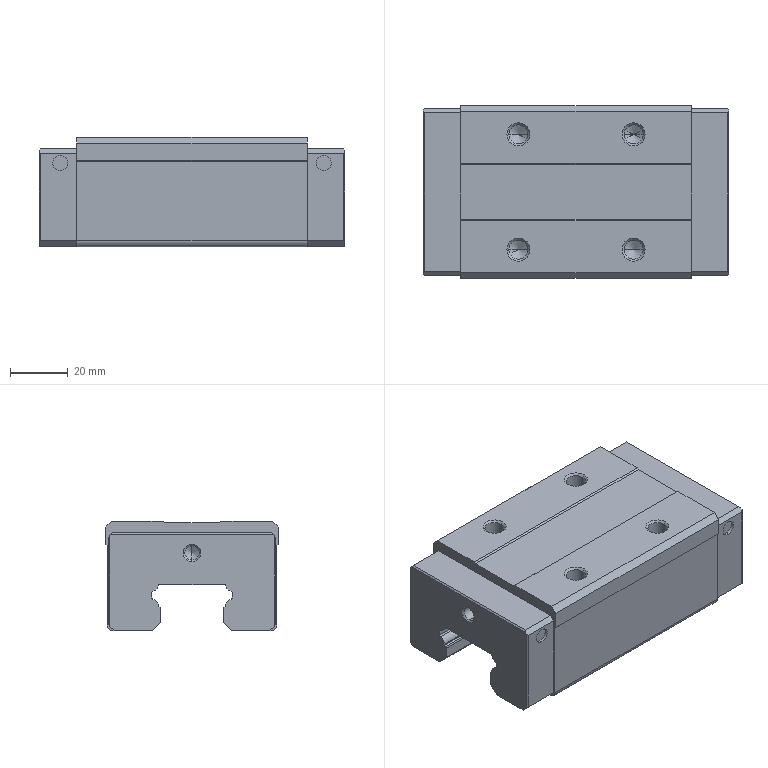Part | SolidWorks | features BaseBody 1 | 1 solid | 118 faces | box 106 x 60 x 38 mm | volume 186804 mm3 | plane 52 | cylinder 42 | cone 24 | commonest cylinder face diameters 5.2 x8 6.647 x8 0.976 x4 4.917 x4 0.952 x2 0.986 x2